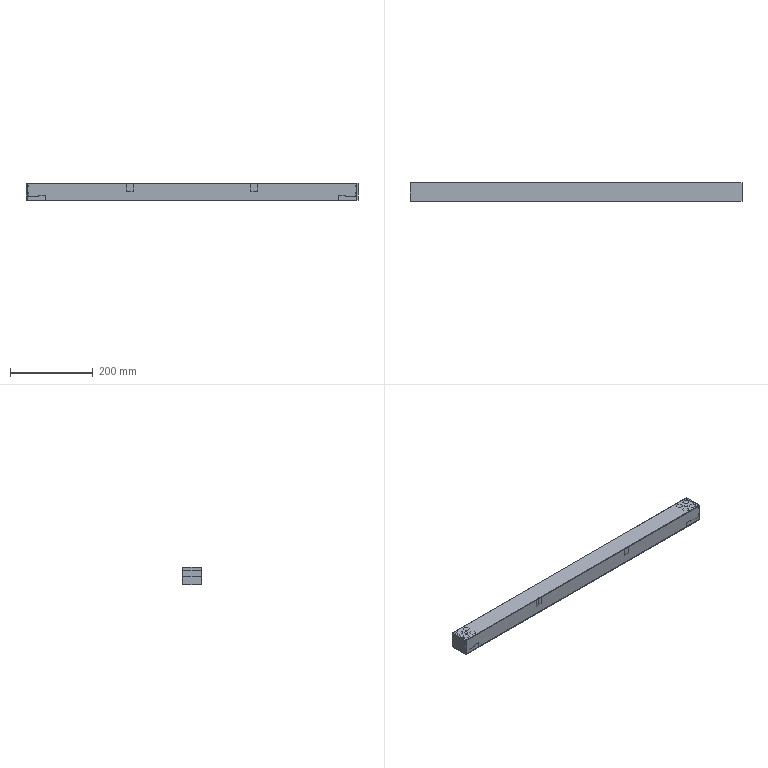NC program | NX | posted with a generic post | part box 801.8 x 45 x 42 mm
Whole program:
N10 G17 G21 G94 G90
(FLOOR_WALL_COPY , TOOL : D63)
N12 T01 M6
N14 G54
N16 G17 G0 G90 X-432.4 Y0. S6500 M3
N18 G43 Z30. H1
N20 Z3.
N22 G94 G1 Z0. F1250.
N24 X-429.4
N26 X429.4
N28 X432.4
N30 Z3.
N32 G0 Z30.
N34 M5
(ZLEVEL_PROFILE_COPY_2 , TOOL : D12)
N36 T20 M6
N38 G54
N40 G17 G0 G90 X406.17 Y33.444 S8000 M3
N42 G43 Z30. H20
N44 Z-1.
N46 G94 G1 X404.596 Y32.535 F3500.
N48 G3 X403.996 Y31.496 R1.2
N50 G1 Y23.409
N52 X404. Y22.53
N54 Y-17.131
N56 X403.996 Y-17.184
N58 Y-31.496
N60 G3 X404.596 Y-32.535 R1.2
N62 G1 X406.17 Y-33.444
N64 G0 Z-2.
N66 G1 X404.596 Y-32.535
N68 G2 X403.996 Y-31.496 R1.2
N70 G1 Y-17.184
N72 X404. Y-17.131
N74 Y22.53
N76 X403.996 Y23.409
N78 Y31.496
N80 G2 X404.596 Y32.535 R1.2
N82 G1 X406.171 Y33.444
N84 G0 Z-3.
N86 G1 X404.596 Y32.535
N88 G3 X403.996 Y31.496 R1.2
N90 G1 Y23.409
N92 X404. Y22.53
N94 Y-17.131
N96 X403.996 Y-17.184
N98 Y-31.496
N100 G3 X404.596 Y-32.535 R1.2
N102 G1 X406.171 Y-33.444
N104 G0 Z-4.
N106 G1 X404.596 Y-32.535
N108 G2 X403.996 Y-31.496 R1.2
N110 G1 Y-17.184
N112 X404. Y-17.131
N114 Y22.53
N116 X403.996 Y23.409
N118 Y31.496
N120 G2 X404.596 Y32.535 R1.2
N122 G1 X406.171 Y33.444
N124 G0 Z-5.
N126 G1 X404.596 Y32.535
N128 G3 X403.996 Y31.496 R1.2
N130 G1 Y23.409
N132 X404. Y22.53
N134 Y-17.131
N136 X403.996 Y-17.184
N138 Y-31.496
N140 G3 X404.596 Y-32.535 R1.2
N142 G1 X406.171 Y-33.444
N144 G0 Z-6.
N146 G1 X404.596 Y-32.535
N148 G2 X403.996 Y-31.496 R1.2
N150 G1 Y-17.184
N152 X404. Y-17.131
N154 Y22.53
N156 X403.996 Y23.409
N158 Y31.496
N160 G2 X404.596 Y32.535 R1.2
N162 G1 X406.171 Y33.444
N164 G0 Z-7.
N166 G1 X404.596 Y32.535
N168 G3 X403.996 Y31.496 R1.2
N170 G1 Y23.409
N172 X404. Y22.53
N174 Y-17.131
N176 X403.996 Y-17.184
N178 Y-31.496
N180 G3 X404.596 Y-32.535 R1.2
N182 G1 X406.171 Y-33.444
N184 G0 Z-8.
N186 G1 X404.596 Y-32.535
N188 G2 X403.996 Y-31.496 R1.2
N190 G1 Y-17.184
N192 X404. Y-17.131
N194 Y22.53
N196 X403.996 Y23.409
N198 Y31.496
N200 G2 X404.596 Y32.535 R1.2
N202 G1 X406.171 Y33.444
N204 G0 Z-9.
N206 G1 X404.596 Y32.535
N208 G3 X403.996 Y31.496 R1.2
N210 G1 Y23.409
N212 X404. Y22.53
N214 Y-17.131
N216 X403.996 Y-17.184
N218 Y-31.496
N220 G3 X404.596 Y-32.535 R1.2
N222 G1 X406.171 Y-33.444
N224 G0 Z-10.
N226 G1 X404.596 Y-32.535
N228 G2 X403.996 Y-31.496 R1.2
N230 G1 Y-17.184
N232 X404. Y-17.131
N234 Y22.53
N236 X403.996 Y23.409
N238 Y31.496
N240 G2 X404.596 Y32.535 R1.2
N242 G1 X406.171 Y33.444
N244 G0 Z-11.
N246 G1 X404.597 Y32.535
N248 G3 X403.997 Y31.496 R1.2
N250 G1 Y23.409
N252 X404. Y22.53
N254 Y-17.131
N256 X403.997 Y-17.184
N258 Y-31.496
N260 G3 X404.597 Y-32.535 R1.2
N262 G1 X406.171 Y-33.444
N264 G0 Z-12.
N266 G1 X404.597 Y-32.535
N268 G2 X403.997 Y-31.496 R1.2
N270 G1 Y-17.184
N272 X404. Y-17.131
N274 Y22.53
N276 X403.997 Y23.409
N278 Y31.496
N280 G2 X404.597 Y32.535 R1.2
N282 G1 X406.171 Y33.444
N284 G0 Z-13.
N286 G1 X404.597 Y32.535
N288 G3 X403.997 Y31.496 R1.2
N290 G1 Y23.409
N292 X404. Y22.53
N294 Y-17.131
N296 X403.997 Y-17.184
N298 Y-31.496
N300 G3 X404.597 Y-32.535 R1.2
N302 G1 X406.171 Y-33.444
N304 G0 Z-14.
N306 G1 X404.597 Y-32.535
N308 G2 X403.997 Y-31.496 R1.2
N310 G1 Y-17.184
N312 X404. Y-17.131
N314 Y22.53
N316 X403.997 Y23.409
N318 Y31.496
N320 G2 X404.597 Y32.535 R1.2
N322 G1 X406.171 Y33.444
N324 G0 Z-15.
N326 G1 X404.597 Y32.535
N328 G3 X403.997 Y31.496 R1.2
N330 G1 Y23.409
N332 X404. Y22.53
N334 Y-17.131
N336 X403.997 Y-17.184
N338 Y-31.496
N340 G3 X404.597 Y-32.535 R1.2
N342 G1 X406.171 Y-33.444
N344 G0 Z-16.
N346 G1 X404.597 Y-32.535
N348 G2 X403.997 Y-31.496 R1.2
N350 G1 Y-17.184
N352 X404. Y-17.131
N354 Y22.53
N356 X403.997 Y23.409
N358 Y31.496
N360 G2 X404.597 Y32.535 R1.2
N362 G1 X406.171 Y33.444
N364 G0 X406.172 Z-17.
N366 G1 X404.597 Y32.535
N368 G3 X403.997 Y31.496 R1.2
N370 G1 Y23.409
N372 X404. Y22.53
N374 Y-17.131
N376 X403.997 Y-17.184
N378 Y-31.496
N380 G3 X404.597 Y-32.535 R1.2
N382 G1 X406.171 Y-33.444
N384 G0 X406.172 Z-18.
N386 G1 X404.597 Y-32.535
N388 G2 X403.997 Y-31.496 R1.2
N390 G1 X404. Y-17.131
N392 Y22.53
N394 X403.997 Y23.409
N396 Y31.496
N398 G2 X404.597 Y32.535 R1.2
N400 G1 X406.172 Y33.444
N402 G0 Z-19.
N404 G1 X404.597 Y32.535
N406 G3 X403.997 Y31.496 R1.2
N408 G1 Y23.409
N410 X404. Y22.53
N412 X403.997 Y-17.184
N414 Y-31.496
N416 G3 X404.597 Y-32.535 R1.2
N418 G1 X406.172 Y-33.444
N420 G0 Z-20.
N422 G1 X404.597 Y-32.535
N424 G2 X403.997 Y-31.496 R1.2
N426 G1 X404. Y-17.131
N428 Y22.53
N430 X403.997 Y23.409
N432 Y31.496
N434 G2 X404.597 Y32.535 R1.2
N436 G1 X406.172 Y33.444
N438 G0 Z-21.
N440 G1 X404.597 Y32.535
N442 G3 X403.997 Y31.496 R1.2
N444 G1 Y23.409
N446 X404. Y22.53
N448 X403.997 Y-17.184
N450 Y-31.496
N452 G3 X404.597 Y-32.535 R1.2
N454 G1 X406.172 Y-33.444
N456 G0 Z-22.
N458 G1 X404.597 Y-32.535
N460 G2 X403.997 Y-31.496 R1.2
N462 G1 X404. Y-17.131
N464 Y22.53
N466 X403.997 Y23.409
N468 Y31.496
N470 G2 X404.597 Y32.535 R1.2
N472 G1 X406.172 Y33.444
N474 G0 Z-23.
N476 G1 X404.597 Y32.535
N478 G3 X403.997 Y31.496 R1.2
N480 G1 Y23.409
N482 X404. Y22.53
N484 X403.997 Y-17.184
N486 Y-31.496
N488 G3 X404.597 Y-32.535 R1.2
N490 G1 X406.172 Y-33.444
N492 G0 Z-24.
N494 G1 X404.597 Y-32.535
N496 G2 X403.997 Y-31.496 R1.2
N498 G1 X404. Y-17.131
N500 Y22.53
N502 X403.998 Y23.409
N504 X403.997 Y31.496
N506 G2 X404.597 Y32.535 R1.2
N508 G1 X406.172 Y33.444
N510 G0 Z-25.
N512 G1 X404.598 Y32.535
N514 G3 X403.998 Y31.496 R1.2
N516 G1 Y23.409
N518 X404. Y22.53
N520 X403.998 Y-17.184
N522 Y-31.496
N524 G3 X404.598 Y-32.535 R1.2
N526 G1 X406.172 Y-33.444
N528 G0 Z-26.
N530 G1 X404.598 Y-32.535
N532 G2 X403.998 Y-31.496 R1.2
N534 G1 X404. Y-17.131
N536 Y22.53
N538 X403.998 Y23.409
N540 Y31.496
N542 G2 X404.598 Y32.535 R1.2
N544 G1 X406.172 Y33.444
N546 G0 Z-27.
N548 G1 X404.598 Y32.535
N550 G3 X403.998 Y31.496 R1.2
N552 G1 Y23.409
N554 X404. Y22.53
N556 X403.998 Y-17.184
N558 Y-31.496
N560 G3 X404.598 Y-32.535 R1.2
N562 G1 X406.172 Y-33.444
N564 G0 Z-28.
N566 G1 X404.598 Y-32.535
N568 G2 X403.998 Y-31.496 R1.2
N570 G1 X404. Y-17.131
N572 Y22.53
N574 X403.998 Y23.409
N576 Y31.496
N578 G2 X404.598 Y32.535 R1.2
N580 G1 X406.172 Y33.444
N582 G0 Z-29.
N584 G1 X404.598 Y32.535
N586 G3 X403.998 Y31.496 R1.2
N588 G1 Y23.409
N590 X404. Y22.53
N592 X403.998 Y-17.184
N594 Y-31.496
N596 G3 X404.598 Y-32.535 R1.2
N598 G1 X406.172 Y-33.444
N600 G0 Z-30.
N602 G1 X404.598 Y-32.535
N604 G2 X403.998 Y-31.496 R1.2
N606 G1 X404. Y-17.131
N608 Y22.53
N610 X403.998 Y31.496
N612 G2 X404.598 Y32.536 R1.2
N614 G1 X406.172 Y33.445
N616 G0 Z-31.
N618 G1 X404.598 Y32.536
N620 G3 X403.998 Y31.496 R1.2
N622 G1 X404. Y22.53
N624 X403.998 Y-17.184
N626 Y-31.496
N628 G3 X404.598 Y-32.535 R1.2
N630 G1 X406.172 Y-33.444
N632 G0 Z-32.
N634 G1 X404.598 Y-32.535
N636 G2 X403.998 Y-31.496 R1.2
N638 G1 X404. Y-17.131
N640 Y22.53
N642 X403.998 Y31.496
N644 G2 X404.598 Y32.536 R1.2
N646 G1 X406.172 Y33.445
N648 G0 Z-33.
N650 G1 X404.598 Y32.536
N652 G3 X403.998 Y31.496 R1.2
N654 G1 X404. Y22.53
N656 Y-17.131
N658 X403.998 Y-31.496
N660 G3 X404.598 Y-32.535 R1.2
N662 G1 X406.172 Y-33.445
N664 G0 X406.173 Z-34.
N666 G1 X404.598 Y-32.535
N668 G2 X403.998 Y-31.496 R1.2
N670 G1 X404. Y-17.131
N672 Y22.53
N674 X403.998 Y31.496
N676 G2 X404.598 Y32.536 R1.2
N678 G1 X406.173 Y33.445
N680 G0 Z-35.
N682 G1 X404.598 Y32.536
N684 G3 X403.998 Y31.496 R1.2
N686 G1 X404. Y22.53
N688 Y-17.131
N690 X403.998 Y-31.496
N692 G3 X404.598 Y-32.535 R1.2
N694 G1 X406.173 Y-33.445
N696 G0 Z-36.
N698 G1 X404.598 Y-32.535
N700 G2 X403.998 Y-31.496 R1.2
N702 G1 X404. Y-17.131
N704 Y22.53
N706 X403.998 Y31.496
N708 G2 X404.598 Y32.536 R1.2
N710 G1 X406.173 Y33.445
N712 G0 Z-37.
N714 G1 X404.598 Y32.536
N716 G3 X403.998 Y31.496 R1.2
N718 G1 X404. Y22.53
N720 Y-17.131
N722 X403.998 Y-31.496
N724 G3 X404.598 Y-32.536 R1.2
N726 G1 X406.173 Y-33.445
N728 G0 Z-38.
N730 G1 X404.598 Y-32.536
N732 G2 X403.999 Y-31.496 R1.2
N734 G1 X404. Y-17.131
N736 Y22.53
N738 X403.999 Y31.496
N740 G2 X404.598 Y32.536 R1.2
N742 G1 X406.173 Y33.445
N744 G0 Z-39.
N746 G1 X404.598 Y32.536
N748 G3 X403.999 Y31.496 R1.2
N750 G1 X404. Y22.53
N752 Y-17.131
N754 X403.999 Y-31.496
N756 G3 X404.599 Y-32.536 R1.2
N758 G1 X406.173 Y-33.445
N760 G0 Z-40.
N762 G1 X404.599 Y-32.536
N764 G2 X403.999 Y-31.496 R1.2
N766 G1 X404. Y-17.131
N768 Y22.53
N770 X403.999 Y31.496
N772 G2 X404.599 Y32.536 R1.2
N774 G1 X406.173 Y33.445
N776 G0 Z30.
N778 X-406.17 Y-33.444
N780 Z-1.
N782 G1 X-404.596 Y-32.535
N784 G3 X-403.996 Y-31.496 R1.2
N786 G1 Y-17.184
N788 X-404. Y-17.131
N790 Y22.5
N792 X-403.972 Y23.088
N794 X-403.996 Y23.143
N796 Y31.496
N798 G3 X-404.596 Y32.535 R1.2
N800 G1 X-406.17 Y33.444
N802 G0 Z-2.
N804 G1 X-404.596 Y32.535
N806 G2 X-403.996 Y31.496 R1.2
N808 G1 Y23.143
N810 X-403.972 Y23.088
N812 X-404. Y22.5
N814 Y-17.131
N816 X-403.996 Y-17.184
N818 Y-31.496
N820 G2 X-404.596 Y-32.535 R1.2
N822 G1 X-406.171 Y-33.444
N824 G0 Z-3.
N826 G1 X-404.596 Y-32.535
N828 G3 X-403.996 Y-31.496 R1.2
N830 G1 Y-17.184
N832 X-404. Y-17.131
N834 Y22.5
N836 X-403.972 Y23.088
N838 X-403.996 Y23.143
N840 Y31.496
N842 G3 X-404.596 Y32.535 R1.2
N844 G1 X-406.171 Y33.444
N846 G0 Z-4.
N848 G1 X-404.596 Y32.535
N850 G2 X-403.996 Y31.496 R1.2
N852 G1 Y23.143
N854 X-403.972 Y23.088
N856 X-404. Y22.5
N858 Y-17.131
N860 X-403.996 Y-17.184
N862 Y-31.496
N864 G2 X-404.596 Y-32.535 R1.2
N866 G1 X-406.171 Y-33.444
N868 G0 Z-5.
N870 G1 X-404.596 Y-32.535
N872 G3 X-403.996 Y-31.496 R1.2
N874 G1 Y-17.184
N876 X-404. Y-17.131
N878 Y22.5
N880 X-403.972 Y23.088
N882 X-403.996 Y23.143
N884 Y31.496
N886 G3 X-404.596 Y32.535 R1.2
N888 G1 X-406.171 Y33.444
N890 G0 Z-6.
N892 G1 X-404.596 Y32.535
N894 G2 X-403.996 Y31.496 R1.2
N896 G1 Y23.143
N898 X-403.972 Y23.088
N900 X-404. Y22.5
N902 Y-17.131
N904 X-403.996 Y-17.184
N906 Y-31.496
N908 G2 X-404.596 Y-32.535 R1.2
N910 G1 X-406.171 Y-33.444
N912 G0 Z-7.
N914 G1 X-404.596 Y-32.535
N916 G3 X-403.996 Y-31.496 R1.2
N918 G1 Y-17.184
N920 X-404. Y-17.131
N922 Y22.5
N924 X-403.972 Y23.088
N926 X-403.996 Y23.143
N928 Y31.496
N930 G3 X-404.596 Y32.535 R1.2
N932 G1 X-406.171 Y33.444
N934 G0 Z-8.
N936 G1 X-404.596 Y32.535
N938 G2 X-403.996 Y31.496 R1.2
N940 G1 Y23.143
N942 X-403.972 Y23.088
N944 X-404. Y22.5
N946 Y-17.131
N948 X-403.996 Y-17.184
N950 Y-31.496
N952 G2 X-404.596 Y-32.535 R1.2
N954 G1 X-406.171 Y-33.444
N956 G0 Z-9.
N958 G1 X-404.596 Y-32.535
N960 G3 X-403.996 Y-31.496 R1.2
N962 G1 Y-17.184
N964 X-404. Y-17.131
N966 Y22.5
N968 X-403.972 Y23.088
N970 X-403.996 Y23.143
N972 Y31.496
N974 G3 X-404.596 Y32.535 R1.2
N976 G1 X-406.171 Y33.444
N978 G0 Z-10.
N980 G1 X-404.596 Y32.535
N982 G2 X-403.996 Y31.496 R1.2
N984 G1 Y23.143
N986 X-403.972 Y23.088
N988 X-404. Y22.5
N990 Y-17.131
N992 X-403.996 Y-17.184
N994 Y-31.496
N996 G2 X-404.596 Y-32.535 R1.2
N998 G1 X-406.171 Y-33.444
N1000 G0 Z-11.
N1002 G1 X-404.597 Y-32.535
N1004 G3 X-403.997 Y-31.496 R1.2
N1006 G1 Y-17.184
N1008 X-404. Y-17.131
N1010 Y22.5
N1012 X-403.972 Y23.088
N1014 X-403.997 Y23.143
N1016 Y31.496
N1018 G3 X-404.597 Y32.535 R1.2
N1020 G1 X-406.171 Y33.444
N1022 G0 Z-12.
N1024 G1 X-404.597 Y32.535
N1026 G2 X-403.997 Y31.496 R1.2
N1028 G1 Y23.143
N1030 X-403.972 Y23.088
N1032 X-404. Y22.5
N1034 Y-17.131
N1036 X-403.997 Y-17.184
N1038 Y-31.496
N1040 G2 X-404.597 Y-32.535 R1.2
N1042 G1 X-406.171 Y-33.444
N1044 G0 Z-13.
N1046 G1 X-404.597 Y-32.535
N1048 G3 X-403.997 Y-31.496 R1.2
N1050 G1 Y-17.184
N1052 X-404. Y-17.131
N1054 Y22.5
N1056 X-403.972 Y23.088
N1058 X-403.997 Y23.143
N1060 Y31.496
N1062 G3 X-404.597 Y32.535 R1.2
N1064 G1 X-406.171 Y33.444
N1066 G0 Z-14.
N1068 G1 X-404.597 Y32.535
N1070 G2 X-403.997 Y31.496 R1.2
N1072 G1 Y23.143
N1074 X-403.972 Y23.088
N1076 X-404. Y22.5
N1078 Y-17.131
N1080 X-403.997 Y-17.184
N1082 Y-31.496
N1084 G2 X-404.597 Y-32.535 R1.2
N1086 G1 X-406.171 Y-33.444
N1088 G0 Z-15.
N1090 G1 X-404.597 Y-32.535
N1092 G3 X-403.997 Y-31.496 R1.2
N1094 G1 Y-17.184
N1096 X-404. Y-17.131
N1098 Y22.5
N1100 X-403.972 Y23.088
N1102 X-403.997 Y23.143
N1104 Y31.496
N1106 G3 X-404.597 Y32.535 R1.2
N1108 G1 X-406.171 Y33.444
N1110 G0 Z-16.
N1112 G1 X-404.597 Y32.535
N1114 G2 X-403.997 Y31.496 R1.2
N1116 G1 Y23.143
N1118 X-403.972 Y23.088
N1120 X-404. Y22.5
N1122 Y-17.131
N1124 X-403.997 Y-17.184
N1126 Y-31.496
N1128 G2 X-404.597 Y-32.535 R1.2
N1130 G1 X-406.171 Y-33.444
N1132 G0 X-406.172 Z-17.
N1134 G1 X-404.597 Y-32.535
N1136 G3 X-403.997 Y-31.496 R1.2
N1138 G1 Y-17.184
N1140 X-404. Y-17.131
N1142 Y22.5
N1144 X-403.972 Y23.088
N1146 X-403.997 Y23.143
N1148 Y31.496
N1150 G3 X-404.597 Y32.535 R1.2
N1152 G1 X-406.171 Y33.444
N1154 G0 X-406.172 Z-18.
N1156 G1 X-404.597 Y32.535
N1158 G2 X-403.997 Y31.496 R1.2
N1160 G1 Y23.143
N1162 X-403.972 Y23.088
N1164 X-404. Y22.5
N1166 X-403.997 Y-17.184
N1168 Y-31.496
N1170 G2 X-404.597 Y-32.535 R1.2
N1172 G1 X-406.172 Y-33.444
N1174 G0 Z-19.
N1176 G1 X-404.597 Y-32.535
N1178 G3 X-403.997 Y-31.496 R1.2
N1180 G1 X-404. Y-17.131
N1182 Y22.5
N1184 X-403.972 Y23.088
N1186 X-403.997 Y23.143
N1188 Y31.496
N1190 G3 X-404.597 Y32.535 R1.2
N1192 G1 X-406.172 Y33.444
N1194 G0 Z-20.
N1196 G1 X-404.597 Y32.535
N1198 G2 X-403.997 Y31.496 R1.2
N1200 G1 Y23.143
N1202 X-403.972 Y23.088
N1204 X-404. Y22.5
N1206 X-403.997 Y-17.184
N1208 Y-31.496
N1210 G2 X-404.597 Y-32.535 R1.2
N1212 G1 X-406.172 Y-33.444
N1214 G0 Z-21.
N1216 G1 X-404.597 Y-32.535
N1218 G3 X-403.997 Y-31.496 R1.2
N1220 G1 X-404. Y-17.131
N1222 Y22.5
N1224 X-403.972 Y23.088
N1226 X-403.997 Y23.143
N1228 Y31.496
N1230 G3 X-404.597 Y32.535 R1.2
N1232 G1 X-406.172 Y33.444
N1234 G0 Z-22.
N1236 G1 X-404.597 Y32.535
N1238 G2 X-403.997 Y31.496 R1.2
N1240 G1 Y23.143
N1242 X-403.972 Y23.088
N1244 X-404. Y22.5
N1246 X-403.997 Y-17.184
N1248 Y-31.496
N1250 G2 X-404.597 Y-32.535 R1.2
N1252 G1 X-406.172 Y-33.444
N1254 G0 Z-23.
N1256 G1 X-404.597 Y-32.535
N1258 G3 X-403.997 Y-31.496 R1.2
N1260 G1 X-404. Y-17.131
N1262 Y22.5
N1264 X-403.972 Y23.088
N1266 X-403.997 Y23.143
N1268 Y31.496
N1270 G3 X-404.597 Y32.535 R1.2
N1272 G1 X-406.172 Y33.444
N1274 G0 Z-24.
N1276 G1 X-404.597 Y32.535
N1278 G2 X-403.997 Y31.496 R1.2
N1280 G1 X-403.998 Y23.143
N1282 X-403.972 Y23.088
N1284 X-404. Y22.5
N1286 X-403.998 Y-17.184
N1288 X-403.997 Y-31.496
N1290 G2 X-404.597 Y-32.535 R1.2
N1292 G1 X-406.172 Y-33.444
N1294 G0 Z-25.
N1296 G1 X-404.598 Y-32.535
N1298 G3 X-403.998 Y-31.496 R1.2
N1300 G1 X-404. Y-17.131
N1302 Y22.5
N1304 X-403.972 Y23.088
N1306 X-403.998 Y23.143
N1308 Y31.496
N1310 G3 X-404.598 Y32.535 R1.2
N1312 G1 X-406.172 Y33.444
N1314 G0 Z-26.
N1316 G1 X-404.598 Y32.535
N1318 G2 X-403.998 Y31.496 R1.2
N1320 G1 Y23.143
N1322 X-403.972 Y23.088
N1324 X-404. Y22.5
N1326 X-403.998 Y-17.184
N1328 Y-31.496
N1330 G2 X-404.598 Y-32.535 R1.2
N1332 G1 X-406.172 Y-33.444
N1334 G0 Z-27.
N1336 G1 X-404.598 Y-32.535
N1338 G3 X-403.998 Y-31.496 R1.2
N1340 G1 X-404. Y-17.131
N1342 Y22.5
N1344 X-403.972 Y23.088
N1346 X-403.998 Y23.143
N1348 Y31.496
N1350 G3 X-404.598 Y32.535 R1.2
N1352 G1 X-406.172 Y33.444
N1354 G0 Z-28.
N1356 G1 X-404.598 Y32.535
N1358 G2 X-403.998 Y31.496 R1.2
N1360 G1 Y23.143
N1362 X-403.972 Y23.088
N1364 X-404. Y22.5
N1366 X-403.998 Y-17.184
N1368 Y-31.496
N1370 G2 X-404.598 Y-32.535 R1.2
N1372 G1 X-406.172 Y-33.444
N1374 G0 Z-29.
N1376 G1 X-404.598 Y-32.535
N1378 G3 X-403.998 Y-31.496 R1.2
N1380 G1 X-404. Y-17.131
N1382 Y22.5
N1384 X-403.972 Y23.088
N1386 X-403.998 Y23.143
N1388 Y31.496
N1390 G3 X-404.598 Y32.535 R1.2
N1392 G1 X-406.172 Y33.444
N1394 G0 Z-30.
N1396 G1 X-404.598 Y32.535
N1398 G2 X-403.998 Y31.496 R1.2
N1400 G1 Y23.143
N1402 X-403.972 Y23.088
N1404 X-404. Y22.5
N1406 X-403.998 Y-17.184
N1408 Y-31.496
N1410 G2 X-404.598 Y-32.535 R1.2
N1412 G1 X-406.172 Y-33.444
N1414 G0 Z-31.
N1416 G1 X-404.598 Y-32.535
N1418 G3 X-403.998 Y-31.496 R1.2
N1420 G1 X-404. Y-17.131
N1422 Y22.5
N1424 X-403.972 Y23.088
N1426 X-403.998 Y23.143
N1428 Y31.496
N1430 G3 X-404.598 Y32.535 R1.2
N1432 G1 X-406.172 Y33.444
N1434 G0 Z-32.
N1436 G1 X-404.598 Y32.535
N1438 G2 X-403.998 Y31.496 R1.2
N1440 G1 Y23.143
N1442 X-403.972 Y23.088
N1444 X-404. Y22.5
N1446 X-403.998 Y-17.184
N1448 Y-31.496
N1450 G2 X-404.598 Y-32.535 R1.2
N1452 G1 X-406.173 Y-33.444
N1454 G0 Y-33.445 Z-33.
N1456 G1 X-404.598 Y-32.535
N1458 G3 X-403.998 Y-31.496 R1.2
N1460 G1 X-404. Y-17.131
N1462 Y22.5
N1464 X-403.972 Y23.088
N1466 X-403.998 Y23.143
N1468 Y31.496
N1470 G3 X-404.598 Y32.535 R1.2
N1472 G1 X-406.173 Y33.444
N1474 G0 Z-34.
N1476 G1 X-404.598 Y32.535
N1478 G2 X-403.998 Y31.496 R1.2
N1480 G1 Y23.143
N1482 X-403.972 Y23.088
N1484 X-404. Y22.5
N1486 Y-17.131
N1488 X-403.998 Y-31.496
N1490 G2 X-404.598 Y-32.535 R1.2
N1492 G1 X-406.173 Y-33.445
N1494 G0 Z-35.
N1496 G1 X-404.598 Y-32.535
N1498 G3 X-403.998 Y-31.496 R1.2
N1500 G1 X-404. Y-17.131
N1502 Y22.5
N1504 X-403.972 Y23.088
N1506 X-403.998 Y23.143
N1508 Y31.496
N1510 G3 X-404.598 Y32.535 R1.2
N1512 G1 X-406.173 Y33.444
N1514 G0 Z-36.
N1516 G1 X-404.598 Y32.535
N1518 G2 X-403.998 Y31.496 R1.2
N1520 G1 Y23.143
N1522 X-403.972 Y23.088
N1524 X-404. Y22.5
N1526 Y-17.131
N1528 X-403.998 Y-31.496
N1530 G2 X-404.598 Y-32.535 R1.2
N1532 G1 X-406.173 Y-33.445
N1534 G0 Z-37.
N1536 G1 X-404.598 Y-32.536
N1538 G3 X-403.998 Y-31.496 R1.2
N1540 G1 X-404. Y-17.131
N1542 Y22.5
N1544 X-403.972 Y23.088
N1546 X-403.998 Y23.143
N1548 Y31.496
N1550 G3 X-404.598 Y32.535 R1.2
N1552 G1 X-406.173 Y33.444
N1554 G0 Z-38.
N1556 G1 X-404.599 Y32.535
N1558 G2 X-403.999 Y31.496 R1.2
N1560 G1 Y23.143
N1562 X-403.972 Y23.088
N1564 X-404. Y22.5
N1566 Y-17.131
N1568 X-403.999 Y-31.496
N1570 G2 X-404.598 Y-32.536 R1.2
N1572 G1 X-406.173 Y-33.445
N1574 G0 Z-39.
N1576 G1 X-404.599 Y-32.536
N1578 G3 X-403.999 Y-31.496 R1.2
N1580 G1 X-404. Y-17.131
N1582 Y22.5
N1584 X-403.972 Y23.088
N1586 X-403.999 Y23.143
N1588 Y31.496
N1590 G3 X-404.599 Y32.535 R1.2
N1592 G1 X-406.173 Y33.444
N1594 G0 Z-40.
N1596 G1 X-404.599 Y32.535
N1598 G2 X-403.999 Y31.496 R1.2
N1600 G1 Y23.143
N1602 X-403.972 Y23.088
N1604 X-404. Y22.5
N1606 Y-17.131
N1608 X-403.999 Y-31.496
N1610 G2 X-404.599 Y-32.536 R1.2
N1612 G1 X-406.173 Y-33.445
N1614 G0 Z30.
N1616 M5
(FLOOR_WALL_1_1 , TOOL : D10)
N1618 T10 M6
N1620 G54
N1622 G17 G0 G90 X403.875 Y28.64 S8000 M3
N1624 G43 Z30. H10
N1626 Z-7.4
N1628 G94 G1 Z-8.9 F1000.
N1630 X403.4 Y28.366
N1632 G3 X402.9 Y27.5 R1.
N1634 G1 Y-27.5 F3000.
N1636 X401.902
N1638 Y27.5
N1640 X400.905
N1642 Y-27.5
N1644 X399.907
N1646 Y27.5
N1648 X398.909
N1650 Y-27.5
N1652 X397.912
N1654 Y27.5
N1656 X396.914
N1658 Y-27.5
N1660 X395.916
N1662 Y27.5
N1664 X394.919
N1666 Y-27.5
N1668 X393.921
N1670 Y27.5
N1672 X392.923
N1674 Y-27.5
N1676 X391.926
N1678 Y27.5
N1680 X390.928
N1682 Y-27.5
N1684 X389.93
N1686 Y27.5
N1688 X388.933
N1690 Y-27.5
N1692 X387.935
N1694 Y27.5
N1696 X386.937
N1698 Y-27.5
N1700 X385.94
N1702 Y27.5
N1704 X384.942
N1706 Y-27.5
N1708 X383.944
N1710 Y27.5
N1712 X382.947
N1714 Y-27.5
N1716 X381.949
N1718 Y27.5
N1720 X380.951
N1722 Y-27.5
N1724 X379.953
N1726 Y27.5
N1728 X378.956
N1730 Y-27.5
N1732 X377.958
N1734 Y27.5
N1736 X376.96
N1738 Y-27.5
N1740 X375.963
N1742 Y27.5
N1744 X374.965
N1746 Y-27.5
N1748 X373.967
N1750 Y27.5
N1752 X372.97
N1754 Y-27.5
N1756 X371.972
N1758 Y27.5
N1760 X370.974
N1762 Y-27.5
N1764 X369.977
N1766 Y27.5
N1768 X368.979
N1770 Y-27.5
N1772 X367.981
N1774 Y27.5
N1776 X366.984
N1778 Y-27.5
N1780 X365.986
N1782 Y27.5
N1784 X364.988
N1786 Y-27.5
N1788 X363.991
N1790 Y27.5
N1792 X362.993
N1794 Y-27.5
N1796 X361.995
N1798 Y27.5
N1800 X360.998
N1802 Y-27.5
N1804 X360.
N1806 Y27.5
N1808 G2 X360.5 Y28.366 R1.
N1810 G1 X361.598 Y29.
N1812 Z-7.4
N1814 G0 Z30.
N1816 X-403.875 Y-28.64
N1818 Z-7.4
N1820 G1 Z-8.9 F1000.
N1822 X-403.4 Y-28.366
N1824 G3 X-402.9 Y-27.5 R1.
N1826 G1 Y27.5 F3000.
N1828 X-401.902
N1830 Y-27.5
N1832 X-400.905
N1834 Y27.5
N1836 X-399.907
N1838 Y-27.5
N1840 X-398.909
N1842 Y27.5
N1844 X-397.912
N1846 Y-27.5
N1848 X-396.914
N1850 Y27.5
N1852 X-395.916
N1854 Y-27.5
N1856 X-394.919
N1858 Y27.5
N1860 X-393.921
N1862 Y-27.5
N1864 X-392.923
N1866 Y27.5
N1868 X-391.926
N1870 Y-27.5
N1872 X-390.928
N1874 Y27.5
N1876 X-389.93
N1878 Y-27.5
N1880 X-388.933
N1882 Y27.5
N1884 X-387.935
N1886 Y-27.5
N1888 X-386.937
N1890 Y27.5
N1892 X-385.94
N1894 Y-27.5
N1896 X-384.942
N1898 Y27.5
N1900 X-383.944
N1902 Y-27.5
N1904 X-382.947
N1906 Y27.5
N1908 X-381.949
N1910 Y-27.5
N1912 X-380.951
N1914 Y27.5
N1916 X-379.953
N1918 Y-27.5
N1920 X-378.956
N1922 Y27.5
N1924 X-377.958
N1926 Y-27.5
N1928 X-376.96
N1930 Y27.5
N1932 X-375.963
N1934 Y-27.5
N1936 X-374.965
N1938 Y27.5
N1940 X-373.967
N1942 Y-27.5
N1944 X-372.97
N1946 Y27.5
N1948 X-371.972
N1950 Y-27.5
N1952 X-370.974
N1954 Y27.5
N1956 X-369.977
N1958 Y-27.5
N1960 X-368.979
N1962 Y27.5
N1964 X-367.981
N1966 Y-27.5
N1968 X-366.984
N1970 Y27.5
N1972 X-365.986
N1974 Y-27.5
N1976 X-364.988
N1978 Y27.5
N1980 X-363.991
N1982 Y-27.5
N1984 X-362.993
N1986 Y27.5
N1988 X-361.995
N1990 Y-27.5
N1992 X-360.998
N1994 Y27.5
N1996 X-360.
N1998 Y-27.5
N2000 G2 X-360.5 Y-28.366 R1.
N2002 G1 X-361.598 Y-29.
N2004 Z-7.4
N2006 G0 Z30.
(FLOOR_WALL_1_2 , TOOL : D10)
N2008 X-362.25
N2010 Z-9.
N2012 G1 Z-10.5 F1000.
N2014 Y-22.5
N2016 X-364.5 F3000.
N2018 Y22.5
N2020 X-360.
N2022 Y-22.5
N2024 X-362.25
N2026 Y-29.
N2028 Z-9.
N2030 G0 Z-10.5
N2032 G1 Z-12. F1000.
N2034 Y-22.5
N2036 X-364.5 F3000.
N2038 Y22.5
N2040 X-360.
N2042 Y-22.5
N2044 X-362.25
N2046 Y-29.
N2048 Z-10.5
N2050 G0 Z30.
N2052 X362.25 Y29.
N2054 Z-9.
N2056 G1 Z-10.5 F1000.
N2058 Y22.5
N2060 X364.5 F3000.
N2062 Y-22.5
N2064 X360.
N2066 Y22.5
N2068 X362.25
N2070 Y29.
N2072 Z-9.
N2074 G0 Z-10.5
N2076 G1 Z-12. F1000.
N2078 Y22.5
N2080 X364.5 F3000.
N2082 Y-22.5
N2084 X360.
N2086 Y22.5
N2088 X362.25
N2090 Y29.
N2092 Z-10.5
N2094 G0 Z30.
(FLOOR_WALL_1_1_COPY , TOOL : D10)
N2096 X403.874 Y28.641
N2098 Z-17.
N2100 G1 Z-18.5 F1000.
N2102 X403.397 Y28.366
N2104 G3 X402.897 Y27.5 R1.
N2106 G1 Y-27.5 F3000.
N2108 X401.965
N2110 Y27.5
N2112 X401.032
N2114 Y-27.5
N2116 X400.1
N2118 Y27.5
N2120 G2 X400.6 Y28.366 R1.
N2122 G1 X401.698 Y29.
N2124 Z-17.
N2126 G0 Z30.
N2128 X-403.874 Y-28.641
N2130 Z-17.
N2132 G1 Z-18.5 F1000.
N2134 X-403.397 Y-28.366
N2136 G3 X-402.897 Y-27.5 R1.
N2138 G1 Y27.5 F3000.
N2140 X-401.965
N2142 Y-27.5
N2144 X-401.032
N2146 Y27.5
N2148 X-400.1
N2150 Y-27.5
N2152 G2 X-400.6 Y-28.366 R1.
N2154 G1 X-401.698 Y-29.
N2156 Z-17.
N2158 G0 Z30.
N2160 M5
(DRILLING_COPY_1 , TOOL : D6A45)
N2162 T07 M6
N2164 G54
N2166 G17 G0 G90 X386. Y-11. S3000 M3
N2168 G43 Z30. H7
N2170 G94 G81 G98 Z-10. F200. R-6.
N2172 Y11.
N2174 X375. Y0.
N2176 X364. Y11. Z-13.1 R-9.1
N2178 Y-11.
N2180 X-364.
N2182 Y11.
N2184 X-375. Y0. Z-10. R-6.
N2186 X-386. Y11.
N2188 Y-11.
N2190 G80
N2192 G0 X-386. Y-11. Z30.
N2194 M5
(DRILLING_COPY_COPY_1 , TOOL : 8.5ZT)
N2196 T08 M6
N2198 G54
N2200 G17 G0 G90 X-386. Y-11. S1500 M3
N2202 G43 Z30. H8
N2204 G94 G83 G98 Z-40. F200. Q2. R-6.
N2206 Y11.
N2208 X-364. R-9.1
N2210 Y-11.
N2212 X364.
N2214 Y11.
N2216 X386. R-6.
N2218 Y-11.
N2220 G80
N2222 G0 X386. Y-11. Z30.
N2224 M5
(DRILLING_COPY_COPY_COPY_1 , TOOL : 7.8ZT)
N2226 T12 M6
N2228 G54
N2230 G17 G0 G90 X-375. Y0. S1500 M3
N2232 G43 Z30. H12
N2234 G94 G83 G98 Z-43.843 F200. Q2. R-6.
N2236 X375.
N2238 G80
N2240 G0 X375. Y0. Z30.
N2242 M5
(DRILLING_COPY_COPY_COPY_COPY_1 , TOOL : 8.0JD)
N2244 T13 M6
N2246 G54
N2248 G17 G0 G90 X-375. Y0. S1000 M3
N2250 G43 Z30. H13
N2252 G94 G85 G98 Z-40.5 F50. R-6.
N2254 X375.
N2256 G80
N2258 G0 X375. Y0. Z30.
N2260 M5
(FLOOR_WALL_1_COPY , TOOL : D10JING)
N2262 T11 M6
N2264 G54
N2266 G17 G0 G90 X-400. Y-29. S8000 M3
N2268 G43 Z30. H11
N2270 Z-17.1
N2272 G94 G1 Z-18.6 F1000.
N2274 Y-27.5
N2276 Y27.5 F1200.
N2278 Y29.
N2280 Z-17.1
N2282 G0 Z30.
N2284 X-394.999 Y-29.
N2286 Z-7.5
N2288 G1 Z-9. F1000.
N2290 Y-27.5
N2292 Y27.5 F1200.
N2294 X-389.649
N2296 Y-27.5
N2298 X-384.3
N2300 Y27.5
N2302 X-378.95
N2304 Y-27.5
N2306 X-373.6
N2308 Y27.5
N2310 Y29.
N2312 Z-7.5
N2314 G0 Z30.
N2316 X-364.599 Y-29.
N2318 Z-10.6
N2320 G1 Z-12.1 F1000.
N2322 Y-27.5
N2324 Y27.5 F1200.
N2326 X-359.9
N2328 Y-27.5
N2330 Y-29.
N2332 Z-10.6
N2334 G0 Z30.
N2336 X359.901
N2338 Z-10.6
N2340 G1 Z-12.1 F1000.
N2342 Y-27.5
N2344 Y27.5 F1200.
N2346 X364.6
N2348 Y-27.5
N2350 Y-29.
N2352 Z-10.6
N2354 G0 Z30.
N2356 X369.601
N2358 Z-7.5
N2360 G1 Z-9. F1000.
N2362 Y-27.5
N2364 Y27.5 F1200.
N2366 X374.951
N2368 Y-27.5
N2370 X380.301
N2372 Y27.5
N2374 X385.65
N2376 Y-27.5
N2378 X391.
N2380 Y27.5
N2382 Y29.
N2384 Z-7.5
N2386 G0 Z30.
N2388 X400.
N2390 Z-17.1
N2392 G1 Z-18.6 F1000.
N2394 Y27.5
N2396 Y-27.5 F1200.
N2398 Y-29.
N2400 Z-17.1
N2402 G0 Z30.
(刀补11. , TOOL : D10JING)
N2404 X-400.017 Y-29.098
N2406 Z-17.1
N2408 G1 Z-18.6 F1000.
N2410 G41 X-400. Y-29. D11
N2412 Y-27.5
N2414 Y27.5 F1200.
N2416 Y29.
N2418 G40
N2420 X-400.017 Y29.098
N2422 Z-17.1
N2424 G0 Z30.
N2426 X-364.583
N2428 Z-10.6
N2430 G1 Z-12.1 F1000.
N2432 G41 X-364.6 Y29.
N2434 Y27.5
N2436 Y-27.5 F1200.
N2438 Y-28.5
N2440 G40
N2442 X-364.583 Y-28.598
N2444 X-359.917
N2446 G41 X-359.9 Y-28.5 F1000.
N2448 Y-27.5
N2450 Y27.5 F1200.
N2452 Y29.
N2454 G40
N2456 X-359.917 Y29.098
N2458 Z-10.6
N2460 G0 Z30.
N2462 X359.917
N2464 Z-10.6
N2466 G1 Z-12.1 F1000.
N2468 G41 X359.9 Y29.
N2470 Y27.5
N2472 Y-27.5 F1200.
N2474 Y-28.5
N2476 G40
N2478 X359.917 Y-28.598
N2480 X364.583
N2482 G41 X364.6 Y-28.5 F1000.
N2484 Y-27.5
N2486 Y27.5 F1200.
N2488 Y29.
N2490 G40
N2492 X364.583 Y29.098
N2494 Z-10.6
N2496 G0 Z30.
N2498 X400.017
N2500 Z-17.1
N2502 G1 Z-18.6 F1000.
N2504 G41 X400. Y29.
N2506 Y27.5
N2508 Y-27.5 F1200.
N2510 Y-29.
N2512 G40
N2514 X400.017 Y-29.098
N2516 Z-17.1
N2518 G0 Z30.
N2520 M5
(刀补11_COPY , TOOL : D12JING)
N2522 T21 M6
N2524 G54
N2526 G17 G0 G90 X-406.221 Y-30.827 S8000 M3
N2528 G43 Z30. H21
N2530 Z-23.5
N2532 G94 G1 Z-24.5 F1200.
N2534 G41 X-406.127 Y-30.793 D21
N2536 X-404.498 Y-29.852
N2538 G3 X-403.898 Y-28.813 R1.2
N2540 G1 X-403.899 Y-20.556
N2542 X-403.9 Y-20.541
N2544 Y22.5
N2546 X-403.898 Y22.861
N2548 Y28.813
N2550 G3 X-404.498 Y29.852 R1.2
N2552 G1 X-406.127 Y30.792
N2554 G40
N2556 X-406.221 Y30.826
N2558 Z-23.5
N2560 G0 X-406.222 Y-30.826 Z-39.
N2562 G1 Z-40.
N2564 G41 X-406.128 Y-30.792
N2566 X-404.499 Y-29.852
N2568 G3 X-403.899 Y-28.813 R1.2
N2570 G1 Y-20.999
N2572 X-403.9 Y-20.541
N2574 Y22.5
N2576 X-403.899 Y22.952
N2578 Y28.813
N2580 G3 X-404.499 Y29.852 R1.2
N2582 G1 X-406.128 Y30.792
N2584 G40
N2586 X-406.222 Y30.826
N2588 Z-39.
N2590 G0 Z30.
N2592 M5
(ZLEVEL_PROFILE_COPY_1_COPY_COPY_COPY_COPY_2 , TOOL : D6A45)
N2594 T07 M6
N2596 G54
N2598 G17 G0 G90 X-355.819 Y24.45 S7000 M3
N2600 G43 Z30. H7
N2602 Z-1.
N2604 G94 G1 X-355.42 Y23.759 F1000.
N2606 G3 X-354.901 Y23.459 R0.6
N2608 G1 X354.901
N2610 G2 X355.859 Y22.501 R0.968
N2612 G1 Y-22.501
N2614 G2 X354.901 Y-23.459 R0.968
N2616 G1 X-354.901
N2618 G2 X-355.859 Y-22.501 R0.968
N2620 G1 Y22.501
N2622 G2 X-354.901 Y23.459 R0.968
N2624 G3 X-354.384 Y23.764 R0.6
N2626 G1 X-353.879 Y24.659
N2628 G0 Z30.
(ZLEVEL_PROFILE_COPY_1_COPY_COPY_COPY_COPY_2_COPY , TOOL : D6A45)
N2630 X376.439 Y1.149
N2632 Z-10.
N2634 G1 X375.52 Y2.741
N2636 G3 X375. Y3.041 R0.6
N2638 G1 X374.998
N2640 G3 X371.959 Y-0.002 R3.041
N2642 X375. Y3.041 R-3.041
N2644 X374.48 Y2.741 R0.6
N2646 G1 X373.561 Y1.149
N2648 G0 Z30.
N2650 X384.698 Y-12.637
N2652 Z-10.
N2654 G1 X385.48 Y-13.991
N2656 G3 X386. Y-14.291 R0.6
N2658 G1 X386.004
N2660 G3 X389.291 Y-10.996 R3.291
N2662 X386. Y-14.291 R-3.291
N2664 X386.52 Y-13.991 R0.6
N2666 G1 X387.302 Y-12.637
N2668 G0 Z30.
N2670 X387.637 Y9.698
N2672 Z-10.
N2674 G1 X388.991 Y10.48
N2676 G3 X389.291 Y11. R0.6
N2678 X386. Y14.291 R3.291
N2680 X389.291 Y11. R-3.291
N2682 X388.991 Y11.52 R0.6
N2684 G1 X387.637 Y12.302
N2686 G0 Z30.
N2688 X-373.561 Y1.149
N2690 Z-10.
N2692 G1 X-374.48 Y2.741
N2694 G3 X-375. Y3.041 R0.6
N2696 X-378.041 Y0. R3.041
N2698 X-375. Y3.041 R-3.041
N2700 X-375.52 Y2.741 R0.6
N2702 G1 X-376.439 Y1.149
N2704 G0 Z30.
N2706 X-387.302 Y-12.637
N2708 Z-10.
N2710 G1 X-386.52 Y-13.991
N2712 G3 X-386. Y-14.291 R0.6
N2714 X-382.709 Y-11. R3.291
N2716 X-386. Y-14.291 R-3.291
N2718 X-385.48 Y-13.991 R0.6
N2720 G1 X-384.698 Y-12.637
N2722 G0 Z30.
N2724 X-387.637 Y12.302
N2726 Z-10.
N2728 G1 X-388.991 Y11.52
N2730 G3 X-389.291 Y11. R0.6
N2732 X-386. Y7.709 R3.291
N2734 X-389.291 Y11. R-3.291
N2736 X-388.991 Y10.48 R0.6
N2738 G1 X-387.637 Y9.698
N2740 G0 Z30.
N2742 X-396.951 Y-23.42
N2744 Z-10.
N2746 G1 X-396.259 Y-23.02
N2748 G3 X-395.959 Y-22.501 R0.6
N2750 G1 Y22.501
N2752 G2 X-395. Y23.459 R0.962
N2754 G1 X-369.599
N2756 G2 X-368.641 Y22.501 R0.966
N2758 G1 Y-22.501
N2760 G2 X-369.599 Y-23.459 R0.966
N2762 G1 X-395.
N2764 G2 X-395.959 Y-22.501 R0.962
N2766 G3 X-396.261 Y-21.982 R0.6
N2768 G1 X-397.159 Y-21.469
N2770 G0 Z30.
N2772 X396.951 Y23.42
N2774 Z-10.
N2776 G1 X396.259 Y23.02
N2778 G3 X395.959 Y22.501 R0.6
N2780 G1 Y-22.501
N2782 G2 X395. Y-23.459 R0.962
N2784 G1 X369.599
N2786 G2 X368.641 Y-22.501 R0.966
N2788 G1 Y22.501
N2790 G2 X369.599 Y23.459 R0.966
N2792 G1 X395.
N2794 G2 X395.959 Y22.501 R0.962
N2796 G3 X396.261 Y21.982 R0.6
N2798 G1 X397.159 Y21.469
N2800 G0 Z30.
N2802 M5
N2804 M2